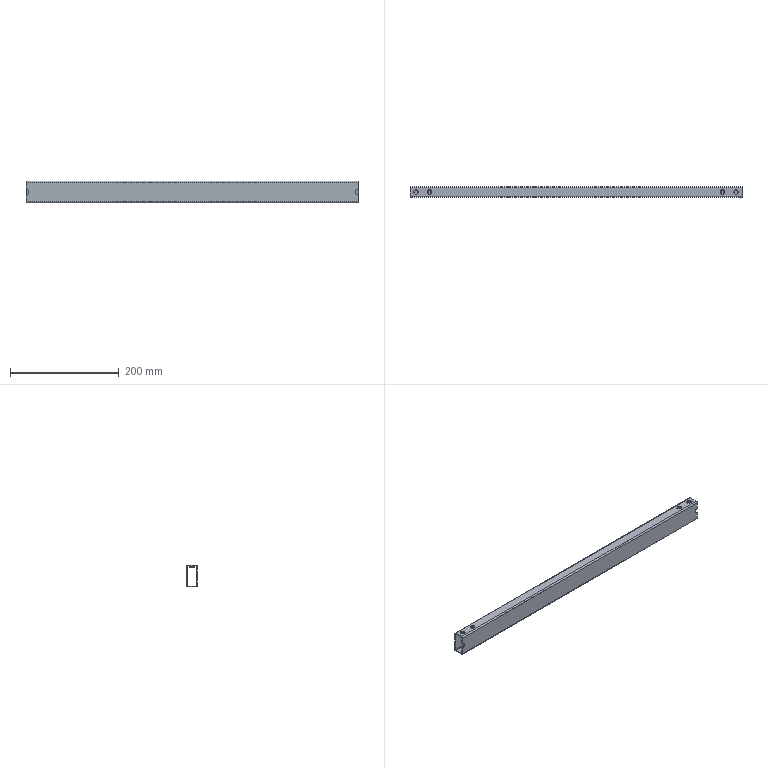Part | STEP file | Q7C0504 | 1 solid | 39 faces | box 610 x 20 x 40 mm | volume 101740 mm3 | cylinder 18 | plane 14 | torus 7 | commonest cylinder face diameters 5 x8 2 x4 8 x3 10 x2 9 x1